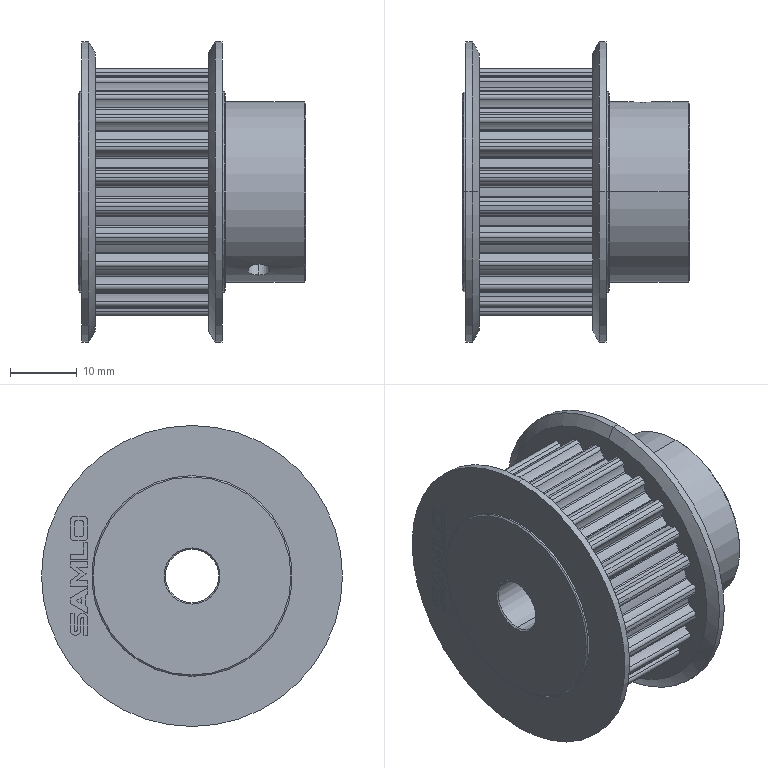Part | SolidWorks | features BaseBody 1 | 1 solid | 316 faces | box 34 x 45 x 45 mm | volume 28395 mm3 | cylinder 243 | plane 59 | cone 14 | commonest cylinder face diameters 1.1 x58 0.5 x56 6.55 x50 33.7 x25 37.24 x24 0.603 x4